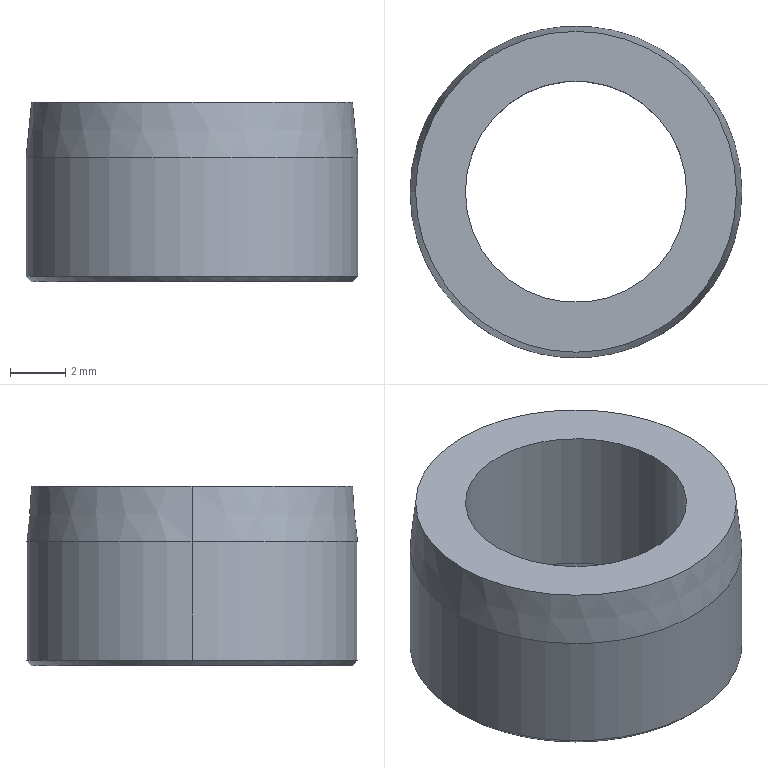Part | STEP file | 1 solid | 12 faces | box 12 x 12 x 6.5 mm | volume 386.592 mm3 | cone 6 | cylinder 4 | plane 2 | commonest cylinder face diameters 8 x2 12 x2
STEP:
#1=CARTESIAN_POINT('',(0.,0.,0.));
#2=DIRECTION('',(0.,0.,1.));
#3=DIRECTION('',(1.,0.,0.));
#4=AXIS2_PLACEMENT_3D('',#1,#2,#3);
#5=CARTESIAN_POINT('',(5.8,0.,6.5));
#6=VERTEX_POINT('',#5);
#7=CARTESIAN_POINT('',(-5.8,0.,6.5));
#8=VERTEX_POINT('',#7);
#9=CARTESIAN_POINT('',(0.,0.,6.5));
#10=DIRECTION('',(0.,0.,1.));
#11=DIRECTION('',(1.,0.,0.));
#12=AXIS2_PLACEMENT_3D('',#9,#10,#11);
#13=CIRCLE('',#12,5.8);
#14=CARTESIAN_POINT('',(0.,0.,6.5));
#15=DIRECTION('',(0.,0.,-1.));
#16=DIRECTION('',(-1.,0.,0.));
#17=AXIS2_PLACEMENT_3D('',#14,#15,#16);
#18=CONICAL_SURFACE('',#17,5.8,0.09967);
#19=CARTESIAN_POINT('',(3.142,0.));
#20=DIRECTION('',(-1.,0.));
#21=VECTOR('',#20,1.);
#22=LINE('',#19,#21);
#23=(GEOMETRIC_REPRESENTATION_CONTEXT(2)PARAMETRIC_REPRESENTATION_CONTEXT()REPRESENTATION_CONTEXT('',''));
#24=DEFINITIONAL_REPRESENTATION('',(#22),#23);
#25=PCURVE('',#18,#24);
#26=CARTESIAN_POINT('',(0.,0.,6.5));
#27=DIRECTION('',(0.,0.,1.));
#28=DIRECTION('',(1.,0.,0.));
#29=AXIS2_PLACEMENT_3D('',#26,#27,#28);
#30=PLANE('',#29);
#31=CARTESIAN_POINT('',(0.,0.));
#32=DIRECTION('',(1.,0.));
#33=AXIS2_PLACEMENT_2D('',#31,#32);
#34=CIRCLE('',#33,5.8);
#35=(GEOMETRIC_REPRESENTATION_CONTEXT(2)PARAMETRIC_REPRESENTATION_CONTEXT()REPRESENTATION_CONTEXT('',''));
#36=DEFINITIONAL_REPRESENTATION('',(#34),#35);
#37=PCURVE('',#30,#36);
#38=SURFACE_CURVE('',#13,(#25,#37),.PCURVE_S1.);
#39=EDGE_CURVE('',#6,#8,#38,.T.);
#40=ORIENTED_EDGE('',*,*,#39,.F.);
#41=CARTESIAN_POINT('',(6.,0.,4.5));
#42=VERTEX_POINT('',#41);
#43=CARTESIAN_POINT('',(5.8,0.,6.5));
#44=DIRECTION('',(0.0995,0.,-0.995));
#45=VECTOR('',#44,1.);
#46=LINE('',#43,#45);
#47=CARTESIAN_POINT('',(3.142,0.));
#48=DIRECTION('',(0.,1.));
#49=VECTOR('',#48,1.);
#50=LINE('',#47,#49);
#51=(GEOMETRIC_REPRESENTATION_CONTEXT(2)PARAMETRIC_REPRESENTATION_CONTEXT()REPRESENTATION_CONTEXT('',''));
#52=DEFINITIONAL_REPRESENTATION('',(#50),#51);
#53=PCURVE('',#18,#52);
#54=CARTESIAN_POINT('',(0.,0.,6.5));
#55=DIRECTION('',(0.,0.,-1.));
#56=DIRECTION('',(-1.,0.,0.));
#57=AXIS2_PLACEMENT_3D('',#54,#55,#56);
#58=CONICAL_SURFACE('',#57,5.8,0.09967);
#59=CARTESIAN_POINT('',(3.142,0.));
#60=DIRECTION('',(0.,1.));
#61=VECTOR('',#60,1.);
#62=LINE('',#59,#61);
#63=(GEOMETRIC_REPRESENTATION_CONTEXT(2)PARAMETRIC_REPRESENTATION_CONTEXT()REPRESENTATION_CONTEXT('',''));
#64=DEFINITIONAL_REPRESENTATION('',(#62),#63);
#65=PCURVE('',#58,#64);
#66=SURFACE_CURVE('',#46,(#53,#65),.PCURVE_S1.);
#67=EDGE_CURVE('',#6,#42,#66,.T.);
#68=ORIENTED_EDGE('',*,*,#67,.T.);
#69=CARTESIAN_POINT('',(-6.,0.,4.5));
#70=VERTEX_POINT('',#69);
#71=CARTESIAN_POINT('',(0.,0.,4.5));
#72=DIRECTION('',(0.,0.,-1.));
#73=DIRECTION('',(1.,0.,0.));
#74=AXIS2_PLACEMENT_3D('',#71,#72,#73);
#75=CIRCLE('',#74,6.);
#76=CARTESIAN_POINT('',(-3.142,2.));
#77=DIRECTION('',(1.,0.));
#78=VECTOR('',#77,1.);
#79=LINE('',#76,#78);
#80=(GEOMETRIC_REPRESENTATION_CONTEXT(2)PARAMETRIC_REPRESENTATION_CONTEXT()REPRESENTATION_CONTEXT('',''));
#81=DEFINITIONAL_REPRESENTATION('',(#79),#80);
#82=PCURVE('',#18,#81);
#83=CARTESIAN_POINT('',(0.,0.,6.5));
#84=DIRECTION('',(0.,0.,-1.));
#85=DIRECTION('',(-1.,0.,0.));
#86=AXIS2_PLACEMENT_3D('',#83,#84,#85);
#87=CYLINDRICAL_SURFACE('',#86,6.);
#88=CARTESIAN_POINT('',(-3.142,2.));
#89=DIRECTION('',(1.,0.));
#90=VECTOR('',#89,1.);
#91=LINE('',#88,#90);
#92=(GEOMETRIC_REPRESENTATION_CONTEXT(2)PARAMETRIC_REPRESENTATION_CONTEXT()REPRESENTATION_CONTEXT('',''));
#93=DEFINITIONAL_REPRESENTATION('',(#91),#92);
#94=PCURVE('',#87,#93);
#95=SURFACE_CURVE('',#75,(#82,#94),.PCURVE_S1.);
#96=EDGE_CURVE('',#70,#42,#95,.T.);
#97=ORIENTED_EDGE('',*,*,#96,.F.);
#98=CARTESIAN_POINT('',(-5.8,0.,6.5));
#99=DIRECTION('',(-0.0995,0.,-0.995));
#100=VECTOR('',#99,1.);
#101=LINE('',#98,#100);
#102=CARTESIAN_POINT('',(0.,0.));
#103=DIRECTION('',(0.,1.));
#104=VECTOR('',#103,1.);
#105=LINE('',#102,#104);
#106=(GEOMETRIC_REPRESENTATION_CONTEXT(2)PARAMETRIC_REPRESENTATION_CONTEXT()REPRESENTATION_CONTEXT('',''));
#107=DEFINITIONAL_REPRESENTATION('',(#105),#106);
#108=PCURVE('',#18,#107);
#109=CARTESIAN_POINT('',(6.283,0.));
#110=DIRECTION('',(0.,1.));
#111=VECTOR('',#110,1.);
#112=LINE('',#109,#111);
#113=(GEOMETRIC_REPRESENTATION_CONTEXT(2)PARAMETRIC_REPRESENTATION_CONTEXT()REPRESENTATION_CONTEXT('',''));
#114=DEFINITIONAL_REPRESENTATION('',(#112),#113);
#115=PCURVE('',#58,#114);
#116=SURFACE_CURVE('',#101,(#108,#115),.PCURVE_S1.);
#117=EDGE_CURVE('',#8,#70,#116,.T.);
#118=ORIENTED_EDGE('',*,*,#117,.F.);
#119=EDGE_LOOP('',(#40,#68,#97,#118));
#120=FACE_BOUND('',#119,.T.);
#121=ADVANCED_FACE('',(#120),#18,.T.);
#122=CARTESIAN_POINT('',(-5.8,0.,0.));
#123=VERTEX_POINT('',#122);
#124=CARTESIAN_POINT('',(5.8,0.,0.));
#125=VERTEX_POINT('',#124);
#126=CARTESIAN_POINT('',(0.,0.,0.));
#127=DIRECTION('',(0.,0.,-1.));
#128=DIRECTION('',(1.,0.,0.));
#129=AXIS2_PLACEMENT_3D('',#126,#127,#128);
#130=CIRCLE('',#129,5.8);
#131=CARTESIAN_POINT('',(0.,0.,0.2));
#132=DIRECTION('',(0.,0.,1.));
#133=DIRECTION('',(1.,0.,0.));
#134=AXIS2_PLACEMENT_3D('',#131,#132,#133);
#135=CONICAL_SURFACE('',#134,6.,0.7854);
#136=CARTESIAN_POINT('',(6.283,-0.2));
#137=DIRECTION('',(-1.,0.));
#138=VECTOR('',#137,1.);
#139=LINE('',#136,#138);
#140=(GEOMETRIC_REPRESENTATION_CONTEXT(2)PARAMETRIC_REPRESENTATION_CONTEXT()REPRESENTATION_CONTEXT('',''));
#141=DEFINITIONAL_REPRESENTATION('',(#139),#140);
#142=PCURVE('',#135,#141);
#143=CARTESIAN_POINT('',(0.,0.,0.));
#144=DIRECTION('',(0.,0.,1.));
#145=DIRECTION('',(1.,0.,0.));
#146=AXIS2_PLACEMENT_3D('',#143,#144,#145);
#147=PLANE('',#146);
#148=CARTESIAN_POINT('',(5.8,0.));
#149=CARTESIAN_POINT('',(5.8,-10.046));
#150=CARTESIAN_POINT('',(-2.9,-5.023));
#151=CARTESIAN_POINT('',(-11.6,0.));
#152=CARTESIAN_POINT('',(-2.9,5.023));
#153=CARTESIAN_POINT('',(5.8,10.046));
#154=CARTESIAN_POINT('',(5.8,0.));
#155=(BOUNDED_CURVE()B_SPLINE_CURVE(2,(#148,#149,#150,#151,#152,#153,#154),.UNSPECIFIED.,.T.,.F.)B_SPLINE_CURVE_WITH_KNOTS((1,2,2,2,2,1),(-2.094,0.,2.094,4.189,6.283,8.378),.UNSPECIFIED.)CURVE()GEOMETRIC_REPRESENTATION_ITEM()RATIONAL_B_SPLINE_CURVE((1.,0.5,1.,0.5,1.,0.5,1.))REPRESENTATION_ITEM(''));
#156=(GEOMETRIC_REPRESENTATION_CONTEXT(2)PARAMETRIC_REPRESENTATION_CONTEXT()REPRESENTATION_CONTEXT('',''));
#157=DEFINITIONAL_REPRESENTATION('',(#155),#156);
#158=PCURVE('',#147,#157);
#159=SURFACE_CURVE('',#130,(#142,#158),.PCURVE_S1.);
#160=EDGE_CURVE('',#123,#125,#159,.T.);
#161=ORIENTED_EDGE('',*,*,#160,.F.);
#162=CARTESIAN_POINT('',(-6.,0.,0.2));
#163=VERTEX_POINT('',#162);
#164=CARTESIAN_POINT('',(-6.,0.,0.2));
#165=DIRECTION('',(-0.7071,0.,0.7071));
#166=VECTOR('',#165,1.);
#167=LINE('',#164,#166);
#168=CARTESIAN_POINT('',(3.142,0.));
#169=DIRECTION('',(0.,1.));
#170=VECTOR('',#169,1.);
#171=LINE('',#168,#170);
#172=(GEOMETRIC_REPRESENTATION_CONTEXT(2)PARAMETRIC_REPRESENTATION_CONTEXT()REPRESENTATION_CONTEXT('',''));
#173=DEFINITIONAL_REPRESENTATION('',(#171),#172);
#174=PCURVE('',#135,#173);
#175=CARTESIAN_POINT('',(0.,0.,0.2));
#176=DIRECTION('',(0.,0.,1.));
#177=DIRECTION('',(1.,0.,0.));
#178=AXIS2_PLACEMENT_3D('',#175,#176,#177);
#179=CONICAL_SURFACE('',#178,6.,0.7854);
#180=CARTESIAN_POINT('',(3.142,0.));
#181=DIRECTION('',(0.,1.));
#182=VECTOR('',#181,1.);
#183=LINE('',#180,#182);
#184=(GEOMETRIC_REPRESENTATION_CONTEXT(2)PARAMETRIC_REPRESENTATION_CONTEXT()REPRESENTATION_CONTEXT('',''));
#185=DEFINITIONAL_REPRESENTATION('',(#183),#184);
#186=PCURVE('',#179,#185);
#187=SURFACE_CURVE('',#167,(#174,#186),.PCURVE_S1.);
#188=EDGE_CURVE('',#123,#163,#187,.T.);
#189=ORIENTED_EDGE('',*,*,#188,.T.);
#190=CARTESIAN_POINT('',(6.,0.,0.2));
#191=VERTEX_POINT('',#190);
#192=CARTESIAN_POINT('',(0.,0.,0.2));
#193=DIRECTION('',(0.,0.,1.));
#194=DIRECTION('',(1.,0.,0.));
#195=AXIS2_PLACEMENT_3D('',#192,#193,#194);
#196=CIRCLE('',#195,6.);
#197=CARTESIAN_POINT('',(0.,0.));
#198=DIRECTION('',(1.,0.));
#199=VECTOR('',#198,1.);
#200=LINE('',#197,#199);
#201=(GEOMETRIC_REPRESENTATION_CONTEXT(2)PARAMETRIC_REPRESENTATION_CONTEXT()REPRESENTATION_CONTEXT('',''));
#202=DEFINITIONAL_REPRESENTATION('',(#200),#201);
#203=PCURVE('',#135,#202);
#204=CARTESIAN_POINT('',(3.142,6.3));
#205=DIRECTION('',(-1.,0.));
#206=VECTOR('',#205,1.);
#207=LINE('',#204,#206);
#208=(GEOMETRIC_REPRESENTATION_CONTEXT(2)PARAMETRIC_REPRESENTATION_CONTEXT()REPRESENTATION_CONTEXT('',''));
#209=DEFINITIONAL_REPRESENTATION('',(#207),#208);
#210=PCURVE('',#87,#209);
#211=SURFACE_CURVE('',#196,(#203,#210),.PCURVE_S1.);
#212=EDGE_CURVE('',#191,#163,#211,.T.);
#213=ORIENTED_EDGE('',*,*,#212,.F.);
#214=CARTESIAN_POINT('',(6.,0.,0.2));
#215=DIRECTION('',(0.7071,0.,0.7071));
#216=VECTOR('',#215,1.);
#217=LINE('',#214,#216);
#218=CARTESIAN_POINT('',(0.,0.));
#219=DIRECTION('',(0.,1.));
#220=VECTOR('',#219,1.);
#221=LINE('',#218,#220);
#222=(GEOMETRIC_REPRESENTATION_CONTEXT(2)PARAMETRIC_REPRESENTATION_CONTEXT()REPRESENTATION_CONTEXT('',''));
#223=DEFINITIONAL_REPRESENTATION('',(#221),#222);
#224=PCURVE('',#135,#223);
#225=CARTESIAN_POINT('',(6.283,0.));
#226=DIRECTION('',(0.,1.));
#227=VECTOR('',#226,1.);
#228=LINE('',#225,#227);
#229=(GEOMETRIC_REPRESENTATION_CONTEXT(2)PARAMETRIC_REPRESENTATION_CONTEXT()REPRESENTATION_CONTEXT('',''));
#230=DEFINITIONAL_REPRESENTATION('',(#228),#229);
#231=PCURVE('',#179,#230);
#232=SURFACE_CURVE('',#217,(#224,#231),.PCURVE_S1.);
#233=EDGE_CURVE('',#125,#191,#232,.T.);
#234=ORIENTED_EDGE('',*,*,#233,.F.);
#235=EDGE_LOOP('',(#161,#189,#213,#234));
#236=FACE_BOUND('',#235,.T.);
#237=ADVANCED_FACE('',(#236),#135,.T.);
#238=CARTESIAN_POINT('',(-4.,0.,1.));
#239=VERTEX_POINT('',#238);
#240=CARTESIAN_POINT('',(-5.,0.,0.));
#241=VERTEX_POINT('',#240);
#242=CARTESIAN_POINT('',(-5.,0.,0.));
#243=DIRECTION('',(-0.7071,0.,-0.7071));
#244=VECTOR('',#243,1.);
#245=LINE('',#242,#244);
#246=CARTESIAN_POINT('',(0.,0.,0.));
#247=DIRECTION('',(0.,0.,-1.));
#248=DIRECTION('',(-1.,0.,0.));
#249=AXIS2_PLACEMENT_3D('',#246,#247,#248);
#250=CONICAL_SURFACE('',#249,5.,0.7854);
#251=CARTESIAN_POINT('',(6.283,0.));
#252=DIRECTION('',(0.,1.));
#253=VECTOR('',#252,1.);
#254=LINE('',#251,#253);
#255=(GEOMETRIC_REPRESENTATION_CONTEXT(2)PARAMETRIC_REPRESENTATION_CONTEXT()REPRESENTATION_CONTEXT('',''));
#256=DEFINITIONAL_REPRESENTATION('',(#254),#255);
#257=PCURVE('',#250,#256);
#258=CARTESIAN_POINT('',(0.,0.,0.));
#259=DIRECTION('',(0.,0.,-1.));
#260=DIRECTION('',(-1.,0.,0.));
#261=AXIS2_PLACEMENT_3D('',#258,#259,#260);
#262=CONICAL_SURFACE('',#261,5.,0.7854);
#263=CARTESIAN_POINT('',(0.,0.));
#264=DIRECTION('',(0.,1.));
#265=VECTOR('',#264,1.);
#266=LINE('',#263,#265);
#267=(GEOMETRIC_REPRESENTATION_CONTEXT(2)PARAMETRIC_REPRESENTATION_CONTEXT()REPRESENTATION_CONTEXT('',''));
#268=DEFINITIONAL_REPRESENTATION('',(#266),#267);
#269=PCURVE('',#262,#268);
#270=SURFACE_CURVE('',#245,(#257,#269),.PCURVE_S1.);
#271=EDGE_CURVE('',#239,#241,#270,.T.);
#272=ORIENTED_EDGE('',*,*,#271,.T.);
#273=CARTESIAN_POINT('',(5.,0.,0.));
#274=VERTEX_POINT('',#273);
#275=CARTESIAN_POINT('',(0.,0.,0.));
#276=DIRECTION('',(0.,0.,1.));
#277=DIRECTION('',(1.,0.,0.));
#278=AXIS2_PLACEMENT_3D('',#275,#276,#277);
#279=CIRCLE('',#278,5.);
#280=CARTESIAN_POINT('',(9.425,0.));
#281=DIRECTION('',(-1.,0.));
#282=VECTOR('',#281,1.);
#283=LINE('',#280,#282);
#284=(GEOMETRIC_REPRESENTATION_CONTEXT(2)PARAMETRIC_REPRESENTATION_CONTEXT()REPRESENTATION_CONTEXT('',''));
#285=DEFINITIONAL_REPRESENTATION('',(#283),#284);
#286=PCURVE('',#250,#285);
#287=CARTESIAN_POINT('',(0.,0.));
#288=DIRECTION('',(1.,0.));
#289=AXIS2_PLACEMENT_2D('',#287,#288);
#290=CIRCLE('',#289,5.);
#291=(GEOMETRIC_REPRESENTATION_CONTEXT(2)PARAMETRIC_REPRESENTATION_CONTEXT()REPRESENTATION_CONTEXT('',''));
#292=DEFINITIONAL_REPRESENTATION('',(#290),#291);
#293=PCURVE('',#147,#292);
#294=SURFACE_CURVE('',#279,(#286,#293),.PCURVE_S1.);
#295=EDGE_CURVE('',#241,#274,#294,.T.);
#296=ORIENTED_EDGE('',*,*,#295,.T.);
#297=CARTESIAN_POINT('',(4.,0.,1.));
#298=VERTEX_POINT('',#297);
#299=CARTESIAN_POINT('',(5.,0.,0.));
#300=DIRECTION('',(0.7071,0.,-0.7071));
#301=VECTOR('',#300,1.);
#302=LINE('',#299,#301);
#303=CARTESIAN_POINT('',(3.142,0.));
#304=DIRECTION('',(0.,1.));
#305=VECTOR('',#304,1.);
#306=LINE('',#303,#305);
#307=(GEOMETRIC_REPRESENTATION_CONTEXT(2)PARAMETRIC_REPRESENTATION_CONTEXT()REPRESENTATION_CONTEXT('',''));
#308=DEFINITIONAL_REPRESENTATION('',(#306),#307);
#309=PCURVE('',#250,#308);
#310=CARTESIAN_POINT('',(3.142,0.));
#311=DIRECTION('',(0.,1.));
#312=VECTOR('',#311,1.);
#313=LINE('',#310,#312);
#314=(GEOMETRIC_REPRESENTATION_CONTEXT(2)PARAMETRIC_REPRESENTATION_CONTEXT()REPRESENTATION_CONTEXT('',''));
#315=DEFINITIONAL_REPRESENTATION('',(#313),#314);
#316=PCURVE('',#262,#315);
#317=SURFACE_CURVE('',#302,(#309,#316),.PCURVE_S1.);
#318=EDGE_CURVE('',#298,#274,#317,.T.);
#319=ORIENTED_EDGE('',*,*,#318,.F.);
#320=CARTESIAN_POINT('',(0.,0.,1.));
#321=DIRECTION('',(0.,0.,-1.));
#322=DIRECTION('',(1.,0.,0.));
#323=AXIS2_PLACEMENT_3D('',#320,#321,#322);
#324=CIRCLE('',#323,4.);
#325=CARTESIAN_POINT('',(3.142,-1.));
#326=DIRECTION('',(1.,0.));
#327=VECTOR('',#326,1.);
#328=LINE('',#325,#327);
#329=(GEOMETRIC_REPRESENTATION_CONTEXT(2)PARAMETRIC_REPRESENTATION_CONTEXT()REPRESENTATION_CONTEXT('',''));
#330=DEFINITIONAL_REPRESENTATION('',(#328),#329);
#331=PCURVE('',#250,#330);
#332=CARTESIAN_POINT('',(0.,0.,6.5));
#333=DIRECTION('',(0.,0.,-1.));
#334=DIRECTION('',(-1.,0.,0.));
#335=AXIS2_PLACEMENT_3D('',#332,#333,#334);
#336=CYLINDRICAL_SURFACE('',#335,4.);
#337=CARTESIAN_POINT('',(3.142,5.5));
#338=DIRECTION('',(1.,0.));
#339=VECTOR('',#338,1.);
#340=LINE('',#337,#339);
#341=(GEOMETRIC_REPRESENTATION_CONTEXT(2)PARAMETRIC_REPRESENTATION_CONTEXT()REPRESENTATION_CONTEXT('',''));
#342=DEFINITIONAL_REPRESENTATION('',(#340),#341);
#343=PCURVE('',#336,#342);
#344=SURFACE_CURVE('',#324,(#331,#343),.PCURVE_S1.);
#345=EDGE_CURVE('',#298,#239,#344,.T.);
#346=ORIENTED_EDGE('',*,*,#345,.T.);
#347=EDGE_LOOP('',(#272,#296,#319,#346));
#348=FACE_BOUND('',#347,.F.);
#349=ADVANCED_FACE('',(#348),#250,.F.);
#350=CARTESIAN_POINT('',(-4.,0.,6.5));
#351=VERTEX_POINT('',#350);
#352=CARTESIAN_POINT('',(-4.,0.,6.5));
#353=DIRECTION('',(0.,0.,-1.));
#354=VECTOR('',#353,1.);
#355=LINE('',#352,#354);
#356=CARTESIAN_POINT('',(6.283,0.));
#357=DIRECTION('',(0.,1.));
#358=VECTOR('',#357,1.);
#359=LINE('',#356,#358);
#360=(GEOMETRIC_REPRESENTATION_CONTEXT(2)PARAMETRIC_REPRESENTATION_CONTEXT()REPRESENTATION_CONTEXT('',''));
#361=DEFINITIONAL_REPRESENTATION('',(#359),#360);
#362=PCURVE('',#336,#361);
#363=CARTESIAN_POINT('',(0.,0.,6.5));
#364=DIRECTION('',(0.,0.,-1.));
#365=DIRECTION('',(-1.,0.,0.));
#366=AXIS2_PLACEMENT_3D('',#363,#364,#365);
#367=CYLINDRICAL_SURFACE('',#366,4.);
#368=CARTESIAN_POINT('',(0.,0.));
#369=DIRECTION('',(0.,1.));
#370=VECTOR('',#369,1.);
#371=LINE('',#368,#370);
#372=(GEOMETRIC_REPRESENTATION_CONTEXT(2)PARAMETRIC_REPRESENTATION_CONTEXT()REPRESENTATION_CONTEXT('',''));
#373=DEFINITIONAL_REPRESENTATION('',(#371),#372);
#374=PCURVE('',#367,#373);
#375=SURFACE_CURVE('',#355,(#362,#374),.PCURVE_S1.);
#376=EDGE_CURVE('',#351,#239,#375,.T.);
#377=ORIENTED_EDGE('',*,*,#376,.T.);
#378=ORIENTED_EDGE('',*,*,#345,.F.);
#379=CARTESIAN_POINT('',(4.,0.,6.5));
#380=VERTEX_POINT('',#379);
#381=CARTESIAN_POINT('',(4.,0.,6.5));
#382=DIRECTION('',(0.,0.,-1.));
#383=VECTOR('',#382,1.);
#384=LINE('',#381,#383);
#385=CARTESIAN_POINT('',(3.142,0.));
#386=DIRECTION('',(0.,1.));
#387=VECTOR('',#386,1.);
#388=LINE('',#385,#387);
#389=(GEOMETRIC_REPRESENTATION_CONTEXT(2)PARAMETRIC_REPRESENTATION_CONTEXT()REPRESENTATION_CONTEXT('',''));
#390=DEFINITIONAL_REPRESENTATION('',(#388),#389);
#391=PCURVE('',#336,#390);
#392=CARTESIAN_POINT('',(3.142,0.));
#393=DIRECTION('',(0.,1.));
#394=VECTOR('',#393,1.);
#395=LINE('',#392,#394);
#396=(GEOMETRIC_REPRESENTATION_CONTEXT(2)PARAMETRIC_REPRESENTATION_CONTEXT()REPRESENTATION_CONTEXT('',''));
#397=DEFINITIONAL_REPRESENTATION('',(#395),#396);
#398=PCURVE('',#367,#397);
#399=SURFACE_CURVE('',#384,(#391,#398),.PCURVE_S1.);
#400=EDGE_CURVE('',#380,#298,#399,.T.);
#401=ORIENTED_EDGE('',*,*,#400,.F.);
#402=CARTESIAN_POINT('',(0.,0.,6.5));
#403=DIRECTION('',(0.,0.,1.));
#404=DIRECTION('',(1.,0.,0.));
#405=AXIS2_PLACEMENT_3D('',#402,#403,#404);
#406=CIRCLE('',#405,4.);
#407=CARTESIAN_POINT('',(9.425,0.));
#408=DIRECTION('',(-1.,0.));
#409=VECTOR('',#408,1.);
#410=LINE('',#407,#409);
#411=(GEOMETRIC_REPRESENTATION_CONTEXT(2)PARAMETRIC_REPRESENTATION_CONTEXT()REPRESENTATION_CONTEXT('',''));
#412=DEFINITIONAL_REPRESENTATION('',(#410),#411);
#413=PCURVE('',#336,#412);
#414=CARTESIAN_POINT('',(0.,0.));
#415=DIRECTION('',(1.,0.));
#416=AXIS2_PLACEMENT_2D('',#414,#415);
#417=CIRCLE('',#416,4.);
#418=(GEOMETRIC_REPRESENTATION_CONTEXT(2)PARAMETRIC_REPRESENTATION_CONTEXT()REPRESENTATION_CONTEXT('',''));
#419=DEFINITIONAL_REPRESENTATION('',(#417),#418);
#420=PCURVE('',#30,#419);
#421=SURFACE_CURVE('',#406,(#413,#420),.PCURVE_S1.);
#422=EDGE_CURVE('',#351,#380,#421,.T.);
#423=ORIENTED_EDGE('',*,*,#422,.F.);
#424=EDGE_LOOP('',(#377,#378,#401,#423));
#425=FACE_BOUND('',#424,.F.);
#426=ADVANCED_FACE('',(#425),#336,.F.);
#427=ORIENTED_EDGE('',*,*,#96,.T.);
#428=CARTESIAN_POINT('',(6.,0.,6.5));
#429=DIRECTION('',(0.,0.,-1.));
#430=VECTOR('',#429,1.);
#431=LINE('',#428,#430);
#432=CARTESIAN_POINT('',(3.142,0.));
#433=DIRECTION('',(0.,1.));
#434=VECTOR('',#433,1.);
#435=LINE('',#432,#434);
#436=(GEOMETRIC_REPRESENTATION_CONTEXT(2)PARAMETRIC_REPRESENTATION_CONTEXT()REPRESENTATION_CONTEXT('',''));
#437=DEFINITIONAL_REPRESENTATION('',(#435),#436);
#438=PCURVE('',#87,#437);
#439=CARTESIAN_POINT('',(0.,0.,6.5));
#440=DIRECTION('',(0.,0.,-1.));
#441=DIRECTION('',(-1.,0.,0.));
#442=AXIS2_PLACEMENT_3D('',#439,#440,#441);
#443=CYLINDRICAL_SURFACE('',#442,6.);
#444=CARTESIAN_POINT('',(3.142,0.));
#445=DIRECTION('',(0.,1.));
#446=VECTOR('',#445,1.);
#447=LINE('',#444,#446);
#448=(GEOMETRIC_REPRESENTATION_CONTEXT(2)PARAMETRIC_REPRESENTATION_CONTEXT()REPRESENTATION_CONTEXT('',''));
#449=DEFINITIONAL_REPRESENTATION('',(#447),#448);
#450=PCURVE('',#443,#449);
#451=SURFACE_CURVE('',#431,(#438,#450),.PCURVE_S1.);
#452=EDGE_CURVE('',#42,#191,#451,.T.);
#453=ORIENTED_EDGE('',*,*,#452,.T.);
#454=ORIENTED_EDGE('',*,*,#212,.T.);
#455=CARTESIAN_POINT('',(-6.,0.,6.5));
#456=DIRECTION('',(0.,0.,-1.));
#457=VECTOR('',#456,1.);
#458=LINE('',#455,#457);
#459=CARTESIAN_POINT('',(0.,0.));
#460=DIRECTION('',(0.,1.));
#461=VECTOR('',#460,1.);
#462=LINE('',#459,#461);
#463=(GEOMETRIC_REPRESENTATION_CONTEXT(2)PARAMETRIC_REPRESENTATION_CONTEXT()REPRESENTATION_CONTEXT('',''));
#464=DEFINITIONAL_REPRESENTATION('',(#462),#463);
#465=PCURVE('',#87,#464);
#466=CARTESIAN_POINT('',(6.283,0.));
#467=DIRECTION('',(0.,1.));
#468=VECTOR('',#467,1.);
#469=LINE('',#466,#468);
#470=(GEOMETRIC_REPRESENTATION_CONTEXT(2)PARAMETRIC_REPRESENTATION_CONTEXT()REPRESENTATION_CONTEXT('',''));
#471=DEFINITIONAL_REPRESENTATION('',(#469),#470);
#472=PCURVE('',#443,#471);
#473=SURFACE_CURVE('',#458,(#465,#472),.PCURVE_S1.);
#474=EDGE_CURVE('',#70,#163,#473,.T.);
#475=ORIENTED_EDGE('',*,*,#474,.F.);
#476=EDGE_LOOP('',(#427,#453,#454,#475));
#477=FACE_BOUND('',#476,.T.);
#478=ADVANCED_FACE('',(#477),#87,.T.);
#479=CARTESIAN_POINT('',(0.,0.,6.5));
#480=DIRECTION('',(0.,0.,1.));
#481=DIRECTION('',(1.,0.,0.));
#482=AXIS2_PLACEMENT_3D('',#479,#480,#481);
#483=CIRCLE('',#482,5.8);
#484=CARTESIAN_POINT('',(0.,0.));
#485=DIRECTION('',(1.,0.));
#486=AXIS2_PLACEMENT_2D('',#484,#485);
#487=CIRCLE('',#486,5.8);
#488=(GEOMETRIC_REPRESENTATION_CONTEXT(2)PARAMETRIC_REPRESENTATION_CONTEXT()REPRESENTATION_CONTEXT('',''));
#489=DEFINITIONAL_REPRESENTATION('',(#487),#488);
#490=PCURVE('',#30,#489);
#491=CARTESIAN_POINT('',(9.425,0.));
#492=DIRECTION('',(-1.,0.));
#493=VECTOR('',#492,1.);
#494=LINE('',#491,#493);
#495=(GEOMETRIC_REPRESENTATION_CONTEXT(2)PARAMETRIC_REPRESENTATION_CONTEXT()REPRESENTATION_CONTEXT('',''));
#496=DEFINITIONAL_REPRESENTATION('',(#494),#495);
#497=PCURVE('',#58,#496);
#498=SURFACE_CURVE('',#483,(#490,#497),.PCURVE_S1.);
#499=EDGE_CURVE('',#8,#6,#498,.T.);
#500=ORIENTED_EDGE('',*,*,#499,.T.);
#501=ORIENTED_EDGE('',*,*,#39,.T.);
#502=EDGE_LOOP('',(#500,#501));
#503=FACE_BOUND('',#502,.T.);
#504=ORIENTED_EDGE('',*,*,#422,.F.);
#505=CARTESIAN_POINT('',(0.,0.,6.5));
#506=DIRECTION('',(0.,0.,1.));
#507=DIRECTION('',(1.,0.,0.));
#508=AXIS2_PLACEMENT_3D('',#505,#506,#507);
#509=CIRCLE('',#508,4.);
#510=CARTESIAN_POINT('',(0.,0.));
#511=DIRECTION('',(1.,0.));
#512=AXIS2_PLACEMENT_2D('',#510,#511);
#513=CIRCLE('',#512,4.);
#514=(GEOMETRIC_REPRESENTATION_CONTEXT(2)PARAMETRIC_REPRESENTATION_CONTEXT()REPRESENTATION_CONTEXT('',''));
#515=DEFINITIONAL_REPRESENTATION('',(#513),#514);
#516=PCURVE('',#30,#515);
#517=CARTESIAN_POINT('',(3.142,0.));
#518=DIRECTION('',(-1.,0.));
#519=VECTOR('',#518,1.);
#520=LINE('',#517,#519);
#521=(GEOMETRIC_REPRESENTATION_CONTEXT(2)PARAMETRIC_REPRESENTATION_CONTEXT()REPRESENTATION_CONTEXT('',''));
#522=DEFINITIONAL_REPRESENTATION('',(#520),#521);
#523=PCURVE('',#367,#522);
#524=SURFACE_CURVE('',#509,(#516,#523),.PCURVE_S1.);
#525=EDGE_CURVE('',#380,#351,#524,.T.);
#526=ORIENTED_EDGE('',*,*,#525,.F.);
#527=EDGE_LOOP('',(#504,#526));
#528=FACE_BOUND('',#527,.T.);
#529=ADVANCED_FACE('',(#503,#528),#30,.T.);
#530=CARTESIAN_POINT('',(0.,0.,0.));
#531=DIRECTION('',(0.,0.,-1.));
#532=DIRECTION('',(1.,0.,0.));
#533=AXIS2_PLACEMENT_3D('',#530,#531,#532);
#534=CIRCLE('',#533,5.8);
#535=CARTESIAN_POINT('',(5.8,0.));
#536=CARTESIAN_POINT('',(5.8,-10.046));
#537=CARTESIAN_POINT('',(-2.9,-5.023));
#538=CARTESIAN_POINT('',(-11.6,0.));
#539=CARTESIAN_POINT('',(-2.9,5.023));
#540=CARTESIAN_POINT('',(5.8,10.046));
#541=CARTESIAN_POINT('',(5.8,0.));
#542=(BOUNDED_CURVE()B_SPLINE_CURVE(2,(#535,#536,#537,#538,#539,#540,#541),.UNSPECIFIED.,.T.,.F.)B_SPLINE_CURVE_WITH_KNOTS((1,2,2,2,2,1),(-2.094,0.,2.094,4.189,6.283,8.378),.UNSPECIFIED.)CURVE()GEOMETRIC_REPRESENTATION_ITEM()RATIONAL_B_SPLINE_CURVE((1.,0.5,1.,0.5,1.,0.5,1.))REPRESENTATION_ITEM(''));
#543=(GEOMETRIC_REPRESENTATION_CONTEXT(2)PARAMETRIC_REPRESENTATION_CONTEXT()REPRESENTATION_CONTEXT('',''));
#544=DEFINITIONAL_REPRESENTATION('',(#542),#543);
#545=PCURVE('',#147,#544);
#546=CARTESIAN_POINT('',(6.283,-0.2));
#547=DIRECTION('',(-1.,0.));
#548=VECTOR('',#547,1.);
#549=LINE('',#546,#548);
#550=(GEOMETRIC_REPRESENTATION_CONTEXT(2)PARAMETRIC_REPRESENTATION_CONTEXT()REPRESENTATION_CONTEXT('',''));
#551=DEFINITIONAL_REPRESENTATION('',(#549),#550);
#552=PCURVE('',#179,#551);
#553=SURFACE_CURVE('',#534,(#545,#552),.PCURVE_S1.);
#554=EDGE_CURVE('',#125,#123,#553,.T.);
#555=ORIENTED_EDGE('',*,*,#554,.T.);
#556=ORIENTED_EDGE('',*,*,#160,.T.);
#557=EDGE_LOOP('',(#555,#556));
#558=FACE_BOUND('',#557,.T.);
#559=ORIENTED_EDGE('',*,*,#295,.T.);
#560=CARTESIAN_POINT('',(0.,0.,0.));
#561=DIRECTION('',(0.,0.,1.));
#562=DIRECTION('',(1.,0.,0.));
#563=AXIS2_PLACEMENT_3D('',#560,#561,#562);
#564=CIRCLE('',#563,5.);
#565=CARTESIAN_POINT('',(0.,0.));
#566=DIRECTION('',(1.,0.));
#567=AXIS2_PLACEMENT_2D('',#565,#566);
#568=CIRCLE('',#567,5.);
#569=(GEOMETRIC_REPRESENTATION_CONTEXT(2)PARAMETRIC_REPRESENTATION_CONTEXT()REPRESENTATION_CONTEXT('',''));
#570=DEFINITIONAL_REPRESENTATION('',(#568),#569);
#571=PCURVE('',#147,#570);
#572=CARTESIAN_POINT('',(3.142,0.));
#573=DIRECTION('',(-1.,0.));
#574=VECTOR('',#573,1.);
#575=LINE('',#572,#574);
#576=(GEOMETRIC_REPRESENTATION_CONTEXT(2)PARAMETRIC_REPRESENTATION_CONTEXT()REPRESENTATION_CONTEXT('',''));
#577=DEFINITIONAL_REPRESENTATION('',(#575),#576);
#578=PCURVE('',#262,#577);
#579=SURFACE_CURVE('',#564,(#571,#578),.PCURVE_S1.);
#580=EDGE_CURVE('',#274,#241,#579,.T.);
#581=ORIENTED_EDGE('',*,*,#580,.T.);
#582=EDGE_LOOP('',(#559,#581));
#583=FACE_BOUND('',#582,.T.);
#584=ADVANCED_FACE('',(#558,#583),#147,.F.);
#585=ORIENTED_EDGE('',*,*,#452,.F.);
#586=CARTESIAN_POINT('',(0.,0.,4.5));
#587=DIRECTION('',(0.,0.,-1.));
#588=DIRECTION('',(1.,0.,0.));
#589=AXIS2_PLACEMENT_3D('',#586,#587,#588);
#590=CIRCLE('',#589,6.);
#591=CARTESIAN_POINT('',(3.142,2.));
#592=DIRECTION('',(1.,0.));
#593=VECTOR('',#592,1.);
#594=LINE('',#591,#593);
#595=(GEOMETRIC_REPRESENTATION_CONTEXT(2)PARAMETRIC_REPRESENTATION_CONTEXT()REPRESENTATION_CONTEXT('',''));
#596=DEFINITIONAL_REPRESENTATION('',(#594),#595);
#597=PCURVE('',#443,#596);
#598=CARTESIAN_POINT('',(3.142,2.));
#599=DIRECTION('',(1.,0.));
#600=VECTOR('',#599,1.);
#601=LINE('',#598,#600);
#602=(GEOMETRIC_REPRESENTATION_CONTEXT(2)PARAMETRIC_REPRESENTATION_CONTEXT()REPRESENTATION_CONTEXT('',''));
#603=DEFINITIONAL_REPRESENTATION('',(#601),#602);
#604=PCURVE('',#58,#603);
#605=SURFACE_CURVE('',#590,(#597,#604),.PCURVE_S1.);
#606=EDGE_CURVE('',#42,#70,#605,.T.);
#607=ORIENTED_EDGE('',*,*,#606,.T.);
#608=ORIENTED_EDGE('',*,*,#474,.T.);
#609=CARTESIAN_POINT('',(0.,0.,0.2));
#610=DIRECTION('',(0.,0.,1.));
#611=DIRECTION('',(1.,0.,0.));
#612=AXIS2_PLACEMENT_3D('',#609,#610,#611);
#613=CIRCLE('',#612,6.);
#614=CARTESIAN_POINT('',(9.425,6.3));
#615=DIRECTION('',(-1.,0.));
#616=VECTOR('',#615,1.);
#617=LINE('',#614,#616);
#618=(GEOMETRIC_REPRESENTATION_CONTEXT(2)PARAMETRIC_REPRESENTATION_CONTEXT()REPRESENTATION_CONTEXT('',''));
#619=DEFINITIONAL_REPRESENTATION('',(#617),#618);
#620=PCURVE('',#443,#619);
#621=CARTESIAN_POINT('',(0.,0.));
#622=DIRECTION('',(1.,0.));
#623=VECTOR('',#622,1.);
#624=LINE('',#621,#623);
#625=(GEOMETRIC_REPRESENTATION_CONTEXT(2)PARAMETRIC_REPRESENTATION_CONTEXT()REPRESENTATION_CONTEXT('',''));
#626=DEFINITIONAL_REPRESENTATION('',(#624),#625);
#627=PCURVE('',#179,#626);
#628=SURFACE_CURVE('',#613,(#620,#627),.PCURVE_S1.);
#629=EDGE_CURVE('',#163,#191,#628,.T.);
#630=ORIENTED_EDGE('',*,*,#629,.T.);
#631=EDGE_LOOP('',(#585,#607,#608,#630));
#632=FACE_BOUND('',#631,.T.);
#633=ADVANCED_FACE('',(#632),#443,.T.);
#634=CARTESIAN_POINT('',(0.,0.,1.));
#635=DIRECTION('',(0.,0.,-1.));
#636=DIRECTION('',(1.,0.,0.));
#637=AXIS2_PLACEMENT_3D('',#634,#635,#636);
#638=CIRCLE('',#637,4.);
#639=CARTESIAN_POINT('',(-3.142,5.5));
#640=DIRECTION('',(1.,0.));
#641=VECTOR('',#640,1.);
#642=LINE('',#639,#641);
#643=(GEOMETRIC_REPRESENTATION_CONTEXT(2)PARAMETRIC_REPRESENTATION_CONTEXT()REPRESENTATION_CONTEXT('',''));
#644=DEFINITIONAL_REPRESENTATION('',(#642),#643);
#645=PCURVE('',#367,#644);
#646=CARTESIAN_POINT('',(-3.142,-1.));
#647=DIRECTION('',(1.,0.));
#648=VECTOR('',#647,1.);
#649=LINE('',#646,#648);
#650=(GEOMETRIC_REPRESENTATION_CONTEXT(2)PARAMETRIC_REPRESENTATION_CONTEXT()REPRESENTATION_CONTEXT('',''));
#651=DEFINITIONAL_REPRESENTATION('',(#649),#650);
#652=PCURVE('',#262,#651);
#653=SURFACE_CURVE('',#638,(#645,#652),.PCURVE_S1.);
#654=EDGE_CURVE('',#239,#298,#653,.T.);
#655=ORIENTED_EDGE('',*,*,#654,.F.);
#656=ORIENTED_EDGE('',*,*,#376,.F.);
#657=ORIENTED_EDGE('',*,*,#525,.F.);
#658=ORIENTED_EDGE('',*,*,#400,.T.);
#659=EDGE_LOOP('',(#655,#656,#657,#658));
#660=FACE_BOUND('',#659,.F.);
#661=ADVANCED_FACE('',(#660),#367,.F.);
#662=ORIENTED_EDGE('',*,*,#580,.T.);
#663=ORIENTED_EDGE('',*,*,#271,.F.);
#664=ORIENTED_EDGE('',*,*,#654,.T.);
#665=ORIENTED_EDGE('',*,*,#318,.T.);
#666=EDGE_LOOP('',(#662,#663,#664,#665));
#667=FACE_BOUND('',#666,.F.);
#668=ADVANCED_FACE('',(#667),#262,.F.);
#669=ORIENTED_EDGE('',*,*,#188,.F.);
#670=ORIENTED_EDGE('',*,*,#554,.F.);
#671=ORIENTED_EDGE('',*,*,#233,.T.);
#672=ORIENTED_EDGE('',*,*,#629,.F.);
#673=EDGE_LOOP('',(#669,#670,#671,#672));
#674=FACE_BOUND('',#673,.T.);
#675=ADVANCED_FACE('',(#674),#179,.T.);
#676=ORIENTED_EDGE('',*,*,#67,.F.);
#677=ORIENTED_EDGE('',*,*,#499,.F.);
#678=ORIENTED_EDGE('',*,*,#117,.T.);
#679=ORIENTED_EDGE('',*,*,#606,.F.);
#680=EDGE_LOOP('',(#676,#677,#678,#679));
#681=FACE_BOUND('',#680,.T.);
#682=ADVANCED_FACE('',(#681),#58,.T.);
#683=CLOSED_SHELL('',(#121,#237,#349,#426,#478,#529,#584,#633,#661,#668,#675,#682));
#684=MANIFOLD_SOLID_BREP('',#683);
#685=(LENGTH_UNIT()NAMED_UNIT(*)SI_UNIT(.MILLI.,.METRE.));
#686=UNCERTAINTY_MEASURE_WITH_UNIT(LENGTH_MEASURE(0.0000001),#685,'','');
#687=(NAMED_UNIT(*)PLANE_ANGLE_UNIT()SI_UNIT($,.RADIAN.));
#688=(NAMED_UNIT(*)SI_UNIT($,.STERADIAN.)SOLID_ANGLE_UNIT());
#689=(GEOMETRIC_REPRESENTATION_CONTEXT(3)GLOBAL_UNCERTAINTY_ASSIGNED_CONTEXT((#686))GLOBAL_UNIT_ASSIGNED_CONTEXT((#685,#687,#688))REPRESENTATION_CONTEXT('',''));
#690=ADVANCED_BREP_SHAPE_REPRESENTATION('',(#4,#684),#689);